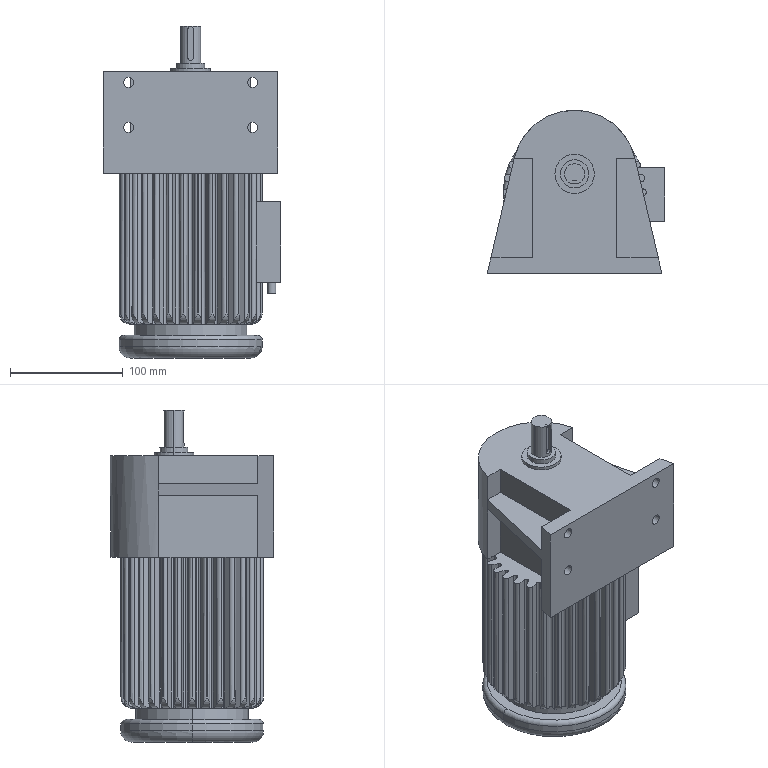Part | STEP file | Motor IPL22-200-30 | 1 solid | 334 faces | box 157.5 x 145 x 294.5 mm | volume 3005281 mm3 | cylinder 185 | plane 114 | torus 35 | commonest cylinder face diameters 6 x82 4 x46 127 x36 9 x8 5 x2 7.101 x2